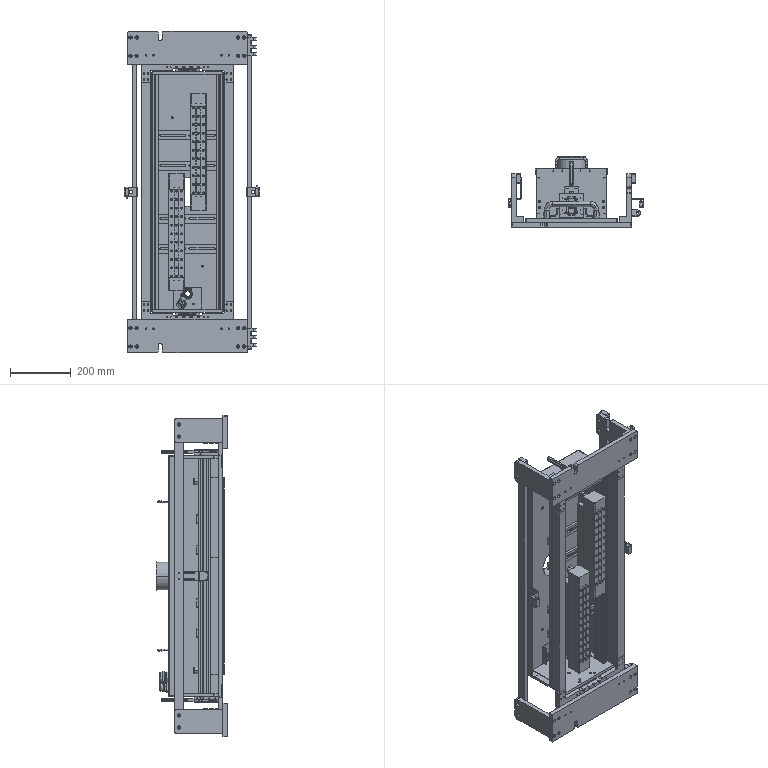Part | SolidWorks | 39 solids | 5599 faces | volume 9622491 mm3 | cylinder 2629 | plane 1809 | cone 1036 | spline 51 | torus 44 | sphere 30 | commonest cylinder face diameters 1 x466 3.3 x210 8 x180 5 x158 4.5 x142 0.659 x131